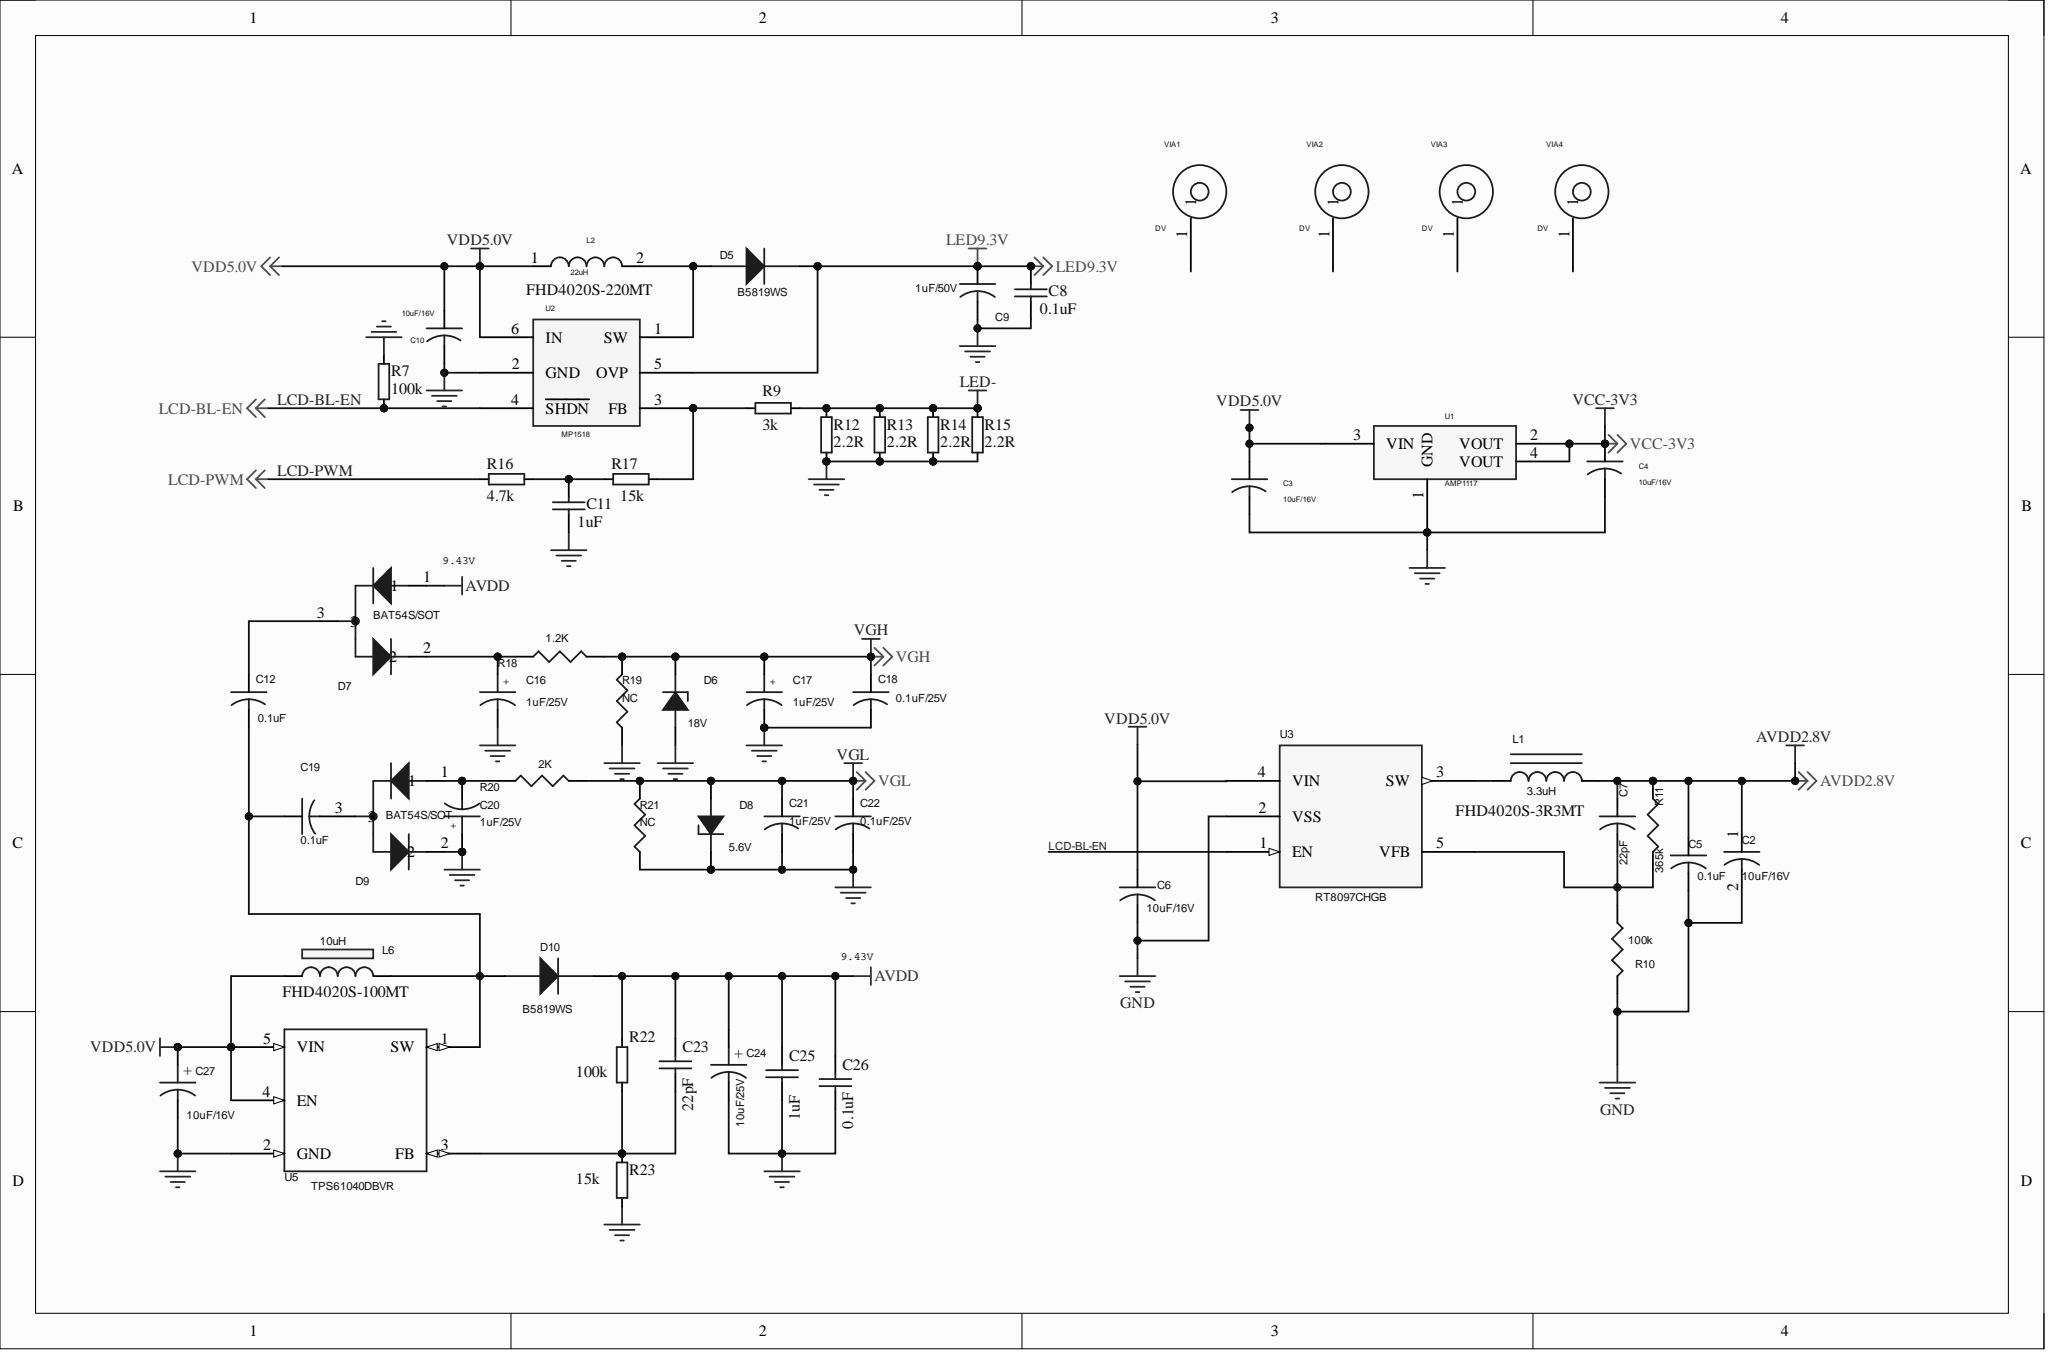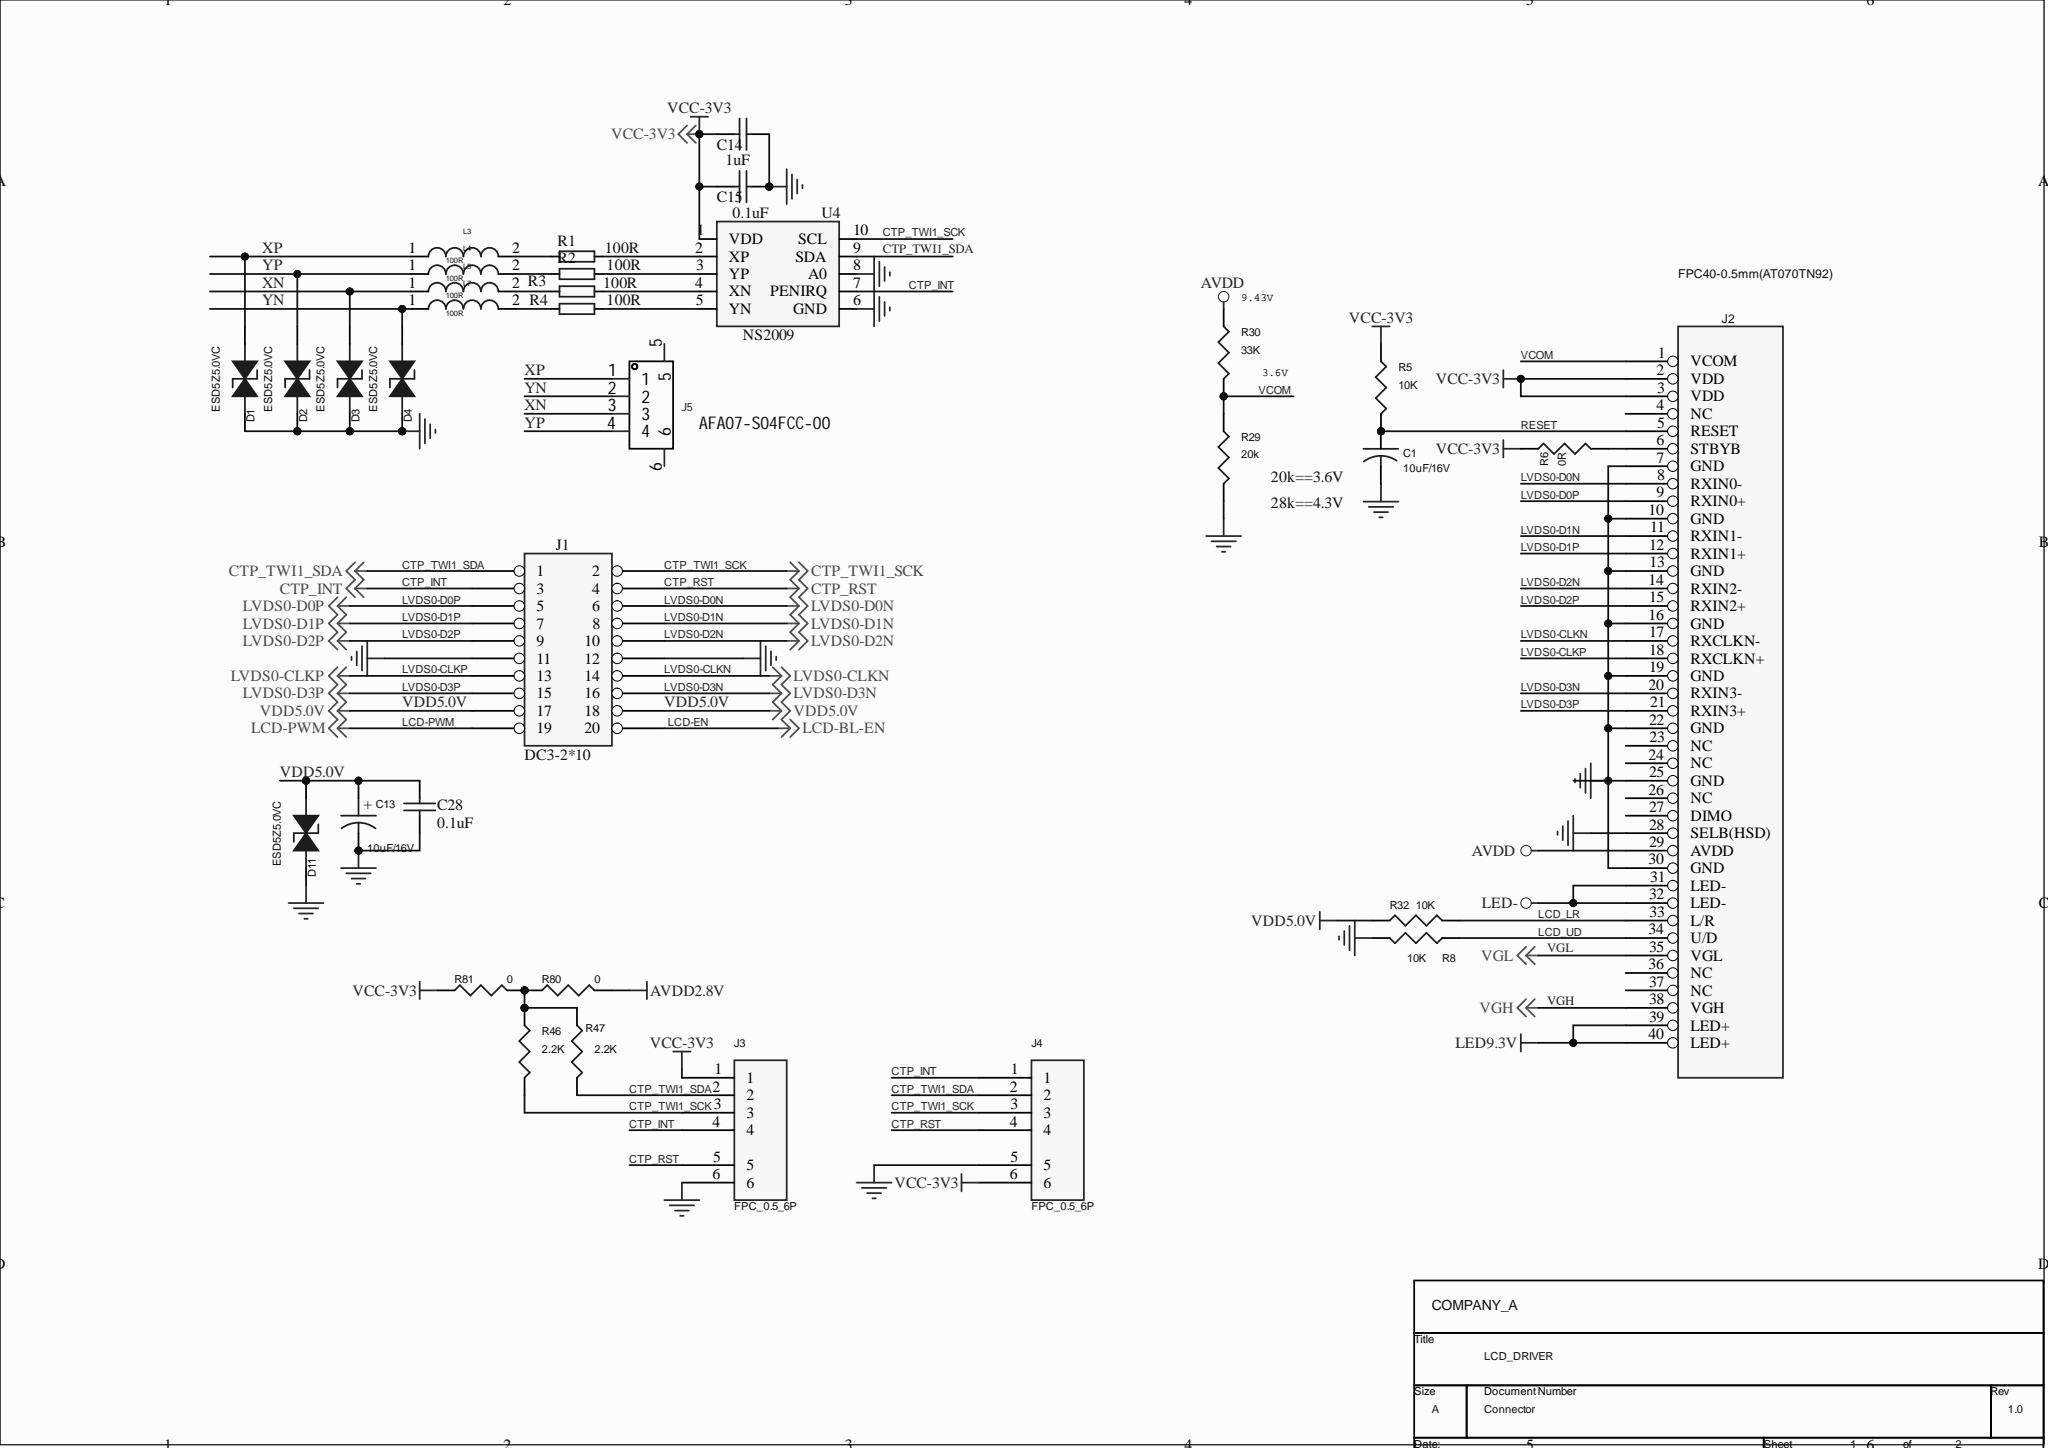Circuit board | Altium Designer | 90 parts | 54 nets
Bill of materials:
Comment,Description,Designator,Footprint,LibRef,Quantity
"10uF/16V","","C1","0603C","C","1"
"10uF/16V","","C2, C3, C4, C6, C10, C13, C27","0805C","CAPACITOR_0, C, CAPACITOR, CAP POL","7"
"0.1uF","[NoValue], Capacitor","C5, C8, C12, C15, C19, C26, C28","0603C","CAPACITOR, CAP, C","7"
"22pF","[NoValue], Capacitor","C7, C23","0603C","CAPACITOR, CAP","2"
"1uF/50V","","C9","0603C","C_Dup1","1"
"1uF","Capacitor","C11, C14, C25","0603C","CAP","3"
"1uF/25V","","C16, C17, C20","0805C","CAP POL","3"
"0.1uF/25V","","C18, C22","0603C","C","2"
"1uF/25V","","C21","0603C","C","1"
"10uF/25V","","C24","0805C","CAP POL","1"
"ESD5Z5.0VC","","D1, D2, D3, D4, D11","SOD-523","1_1.5KE100A","5"
"B5819WS","","D5, D10","SOD-123","BAS21/SOT_1","2"
"18V","","D6","SOD-123","DIODE BREAKDOWN_1","1"
"BAT54S/SOT","","D7, D9","SOT23","BAT54S/SOT","2"
"5.6V","","D8","SOD-123","DIODE BREAKDOWN_1","1"
"DC3-2*10","","J1","DC3-2.0-2*10P","DC3-2*10","1"
"FPC40-0.5mm(AT070TN92)","","J2","FPC40-0.5MM-UP","HEADER 20X2_3","1"
"FPC_0.5_6P","","J3","FPC_0.5_6P_UP","connet_0","1"
"FPC_0.5_6P","","J4","FPC_0.5_6P_DOWN","connet_0","1"
"AFA07-S04FCC-00","","J5","FPC-SMD-1mm4P-RTP","AFC07-S04ECC-00","1"
"3.3uH","","L1","L-SMD-4*4*1.2","INDUCTOR IRON","1"
"22uH","","L2","L-SMD-4*4*1.2","INDUCTOR","1"
"100R","","L3, L4, L5, L7, R1, R2, R3, R4","0603R","INDUCTOR, RES2","8"
"10uH","","L6","L-SMD-4*4*1.2","CHOKE TORROID-FERRITE","1"
"10K","","R5, R8, R32","0603R","R","3"
"0R","","R6","0603R","R","1"
"100k","","R7, R22","0603R","RES2","2"
"3k","","R9","0603R","RES2","1"
"100k","","R10","0603C","R","1"
"365k","","R11","0603R","R","1"
"2.2R","","R12, R13, R14, R15","0805R","RES2","4"
"4.7k","","R16","0603R","RES2","1"
"15k","","R17, R23","0603R","RES2","2"
"1.2K","","R18","0603R","RESISTOR","1"
"NC","","R19, R21","0603R","RESISTOR","2"
"2K","","R20","0603R","RESISTOR","1"
"20k","","R29","0603R","R","1"
"33K","","R30","0603R","R","1"
"2.2K","","R46, R47","0603R","R","2"
"0","","R80, R81","0603R","R","2"
"AMP1117","","U1","SOT223","LM7805/TO_6","1"
"MP1518","","U2","SOT-23-6","PT4110_0","1"
"RT8097CHGB","","U3","SOT23-5","XC9235_0","1"
"NS2009","","U4","MSOP-10","NS2009","1"
"TPS61040DBVR","","U5","SOT-23-5","X9C102/SO_2","1"
"DV","","VIA1, VIA2, VIA3, VIA4","M3","DV_0","4"
Netlist (Protel format):
[
C1
0603C
10uF/16V



]
[
C2
0805C
10uF/16V



]
[
C3
0805C
10uF/16V



]
[
C4
0805C
10uF/16V



]
[
C5
0603C
0.1uF



]
[
C6
0805C
10uF/16V



]
[
C7
0603C
22pF



]
[
C8
0603C
0.1uF



]
[
C9
0603C
1uF/50V



]
[
C10
0805C
10uF/16V



]
[
C11
0603C
1uF



]
[
C12
0603C
0.1uF



]
[
C13
0805C
10uF/16V



]
[
C14
0603C
1uF



]
[
C15
0603C
0.1uF



]
[
C16
0805C
1uF/25V



]
[
C17
0805C
1uF/25V



]
[
C18
0603C
0.1uF/25V



]
[
C19
0603C
0.1uF



]
[
C20
0805C
1uF/25V



]
[
C21
0603C
1uF/25V



]
[
C22
0603C
0.1uF/25V



]
[
C23
0603C
22pF



]
[
C24
0805C
10uF/25V



]
[
C25
0603C
1uF



]
[
C26
0603C
0.1uF



]
[
C27
0805C
10uF/16V



]
[
C28
0603C
0.1uF



]
[
D1
SOD-523
ESD5Z5.0VC



]
[
D2
SOD-523
ESD5Z5.0VC



]
[
D3
SOD-523
ESD5Z5.0VC



]
[
D4
SOD-523
ESD5Z5.0VC



]
[
D5
SOD-123
B5819WS



]
[
D6
SOD-123
18V



]
[
D7
SOT23
BAT54S/SOT



]
[
D8
SOD-123
5.6V



]
[
D9
SOT23
BAT54S/SOT



]
[
D10
SOD-123
B5819WS



]
[
D11
SOD-523
ESD5Z5.0VC



]
[
J1
DC3-2.0-2*10P
DC3-2*10



]
[
J2
FPC40-0.5MM-UP
FPC40-0.5mm(AT070TN92)



]
[
J3
FPC_0.5_6P_UP
FPC_0.5_6P



]
[
J4
FPC_0.5_6P_DOWN
FPC_0.5_6P



]
[
J5
FPC-SMD-1mm4P-RTP
AFA07-S04FCC-00



]
[
L1
L-SMD-4*4*1.2
3.3uH



]
[
L2
L-SMD-4*4*1.2
22uH



]
[
L3
0603R
100R



]
[
L4
0603R
100R



]
[
L5
0603R
100R



]
[
L6
L-SMD-4*4*1.2
10uH



]
[
L7
0603R
100R



]
[
R1
0603R
100R



]
[
R2
0603R
100R



]
[
R3
0603R
100R



]
[
R4
0603R
100R



]
[
R5
0603R
10K



]
[
R6
0603R
0R



]
[
R7
0603R
100k



]
[
R8
0603R
10K



]
[
R9
0603R
3k



]
[
R10
0603C
100k



]
[
R11
0603R
365k



]
[
R12
0805R
2.2R



]
[
R13
0805R
2.2R



]
[
R14
0805R
2.2R



]
[
R15
0805R
2.2R



]
[
R16
0603R
4.7k



]
[
R17
0603R
15k



]
[
R18
0603R
1.2K



]
[
R19
0603R
NC



]
[
R20
0603R
2K



]
[
R21
0603R
NC



]
[
R22
0603R
100k



]
[
R23
0603R
15k



]
[
R29
0603R
20k



]
[
R30
0603R
33K



]
[
R32
0603R
10K



]
[
R46
0603R
2.2K



]
[
R47
0603R
2.2K



]
[
R80
0603R
0



]
[
R81
0603R
0



]
[
U1
SOT223
AMP1117



]
[
U2
SOT-23-6
MP1518



]
[
U3
SOT23-5
RT8097CHGB



]
[
U4
MSOP-10
NS2009



]
[
U5
SOT-23-5
TPS61040DBVR



]
[
VIA1
M3
DV



]
[
VIA2
M3
DV



]
[
VIA3
M3
DV



]
[
VIA4
M3
DV



]
(
YP
D2-1
J5-4
L4-1
)
(
YN
D4-1
J5-2
L7-1
)
(
XP
D1-1
J5-1
L3-1
)
(
XN
D3-1
J5-3
L5-1
)
(
VGL
C21-1
C22-1
D8-1
J2-35
R20-2
R21-2
)
(
VGH
C17-1
C18-1
D6-2
J2-38
R18-2
R19-2
)
(
VDD5.0V
C3-1
C6-1
C10-1
C13-1
C27-1
C28-2
D11-1
J1-17
J1-18
L2-1
L6-1
R32-1
U1-3
U2-6
U3-4
U5-4
U5-5
)
(
VCOM
J2-1
R29-1
R30-2
)
(
VCC-3V3
C4-1
C14-1
C15-1
J2-2
J2-3
J3-1
J4-6
R5-1
R6-1
R81-1
U1-2
U1-4
U4-1
)
(
RESET
C1-1
J2-5
R5-2
)
(
NetR46_1
R46-1
R47-1
R80-1
R81-2
)
(
NetR9_2
R9-2
R17-1
U2-3
)
(
NetR4_2
R4-2
U4-5
)
(
NetR3_2
R3-2
U4-4
)
(
NetR2_2
R2-2
U4-3
)
(
NetR1_2
R1-2
U4-2
)
(
NetL7_2
L7-2
R4-1
)
(
NetL5_2
L5-2
R3-1
)
(
NetL4_2
L4-2
R2-1
)
(
NetL3_2
L3-2
R1-1
)
(
NetL1_1
L1-1
U3-3
)
(
NetJ2_6
J2-6
R6-2
)
(
NetD5_1
D5-1
L2-2
U2-1
)
(
NetC23_2
C23-2
R22-1
R23-2
U5-3
)
(
NetC20_2
C20-2
D9-1
R20-1
)
(
NetC19_2
C19-2
D9-3
)
(
NetC16_1
C16-1
D7-2
R18-1
)
(
NetC12_2
C12-2
C19-1
D10-1
L6-2
U5-1
)
(
NetC12_1
C12-1
D7-3
)
(
NetC11_1
C11-1
R16-1
R17-2
)
(
NetC7_2
C7-2
R10-1
R11-2
U3-5
)
(
LVDS0-D3P
J1-15
J2-21
)
(
LVDS0-D3N
J1-16
J2-20
)
(
LVDS0-D2P
J1-9
J2-15
)
(
LVDS0-D2N
J1-10
J2-14
)
(
LVDS0-D1P
J1-7
J2-12
)
(
LVDS0-D1N
J1-8
J2-11
)
(
LVDS0-D0P
J1-5
J2-9
)
(
LVDS0-D0N
J1-6
J2-8
)
(
LVDS0-CLKP
J1-13
J2-18
)
(
LVDS0-CLKN
J1-14
J2-17
)
(
LED-
J2-31
J2-32
R9-1
R12-1
R13-1
R14-1
R15-1
)
(
LED9.3V
C8-1
C9-1
D5-2
J2-39
J2-40
U2-5
)
(
LCD_UD
J2-34
R8-1
)
(
LCD_LR
J2-33
R32-2
)
(
LCD-PWM
J1-19
R16-2
)
(
LCD-BL-EN
J1-20
R7-2
U2-4
U3-1
)
(
GND
C1-2
C2-2
C3-2
C4-2
C5-2
C6-2
C8-2
C9-2
C10-2
C11-2
C13-2
C14-2
C15-2
C16-2
C17-2
C18-2
C20-1
C21-2
C22-2
C24-2
C25-2
C26-2
C27-2
C28-1
D1-2
D2-2
D3-2
D4-2
D6-1
D8-2
D9-2
D11-2
J1-11
J1-12
J2-7
J2-10
J2-13
J2-16
J2-19
J2-22
J2-25
J2-28
J2-30
J3-6
J4-5
R7-1
R8-2
R10-2
R12-2
R13-2
R14-2
R15-2
R19-1
R21-1
R23-1
R29-2
U1-1
U2-2
U3-2
U4-6
U4-8
U5-2
)
(
CTP_TWI1_SDA
J1-1
J3-2
J4-2
R47-2
U4-9
)
(
CTP_TWI1_SCK
J1-2
J3-3
J4-3
R46-2
U4-10
)
(
CTP_RST
J1-4
J3-5
J4-4
)
(
CTP_INT
J1-3
J3-4
J4-1
U4-7
)
(
AVDD2.8V
C2-1
C5-1
C7-1
L1-2
R11-1
R80-2
)
(
AVDD
C23-1
C24-1
C25-1
C26-1
D7-1
D10-2
J2-29
R22-2
R30-1
)